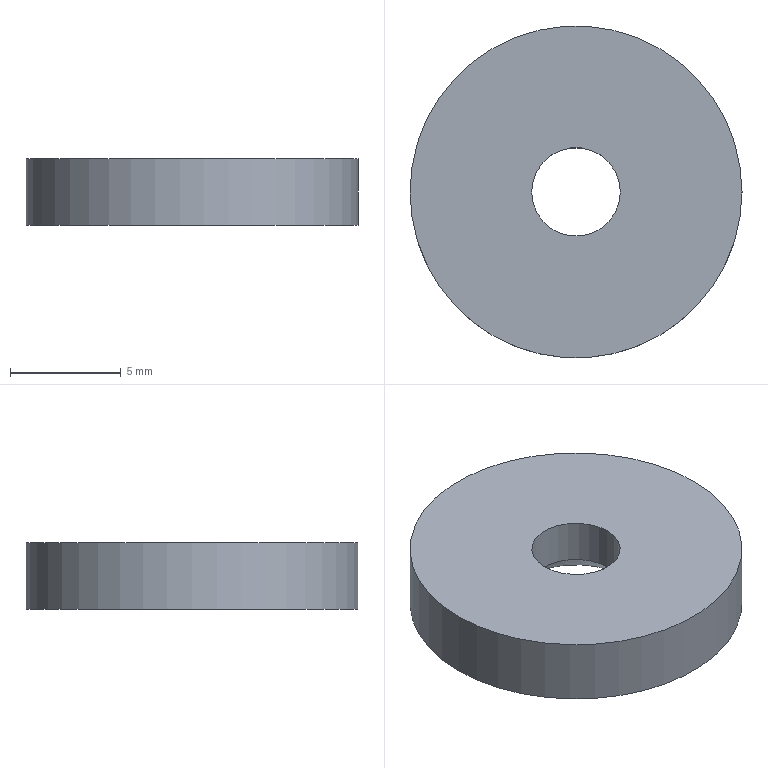Part | NX | features BREP 1, DATUM_CSYS 1 | 1 solid | 5 faces | box 15 x 15 x 3 mm | volume 485.114 mm3 | plane 2 | cylinder 2 | cone 1 | commonest cylinder face diameters 4 x1 15 x1
STEP:
#1=CARTESIAN_POINT('',(7.5,0.,0.));
#2=VERTEX_POINT('',#1);
#3=CARTESIAN_POINT('',(0.,0.,0.));
#4=DIRECTION('',(0.,0.,1.));
#5=DIRECTION('',(1.,0.,0.));
#6=AXIS2_PLACEMENT_3D('',#3,#4,#5);
#7=CIRCLE('',#6,7.5);
#8=EDGE_CURVE('',#2,#2,#7,.T.);
#9=ORIENTED_EDGE('',*,*,#8,.F.);
#10=EDGE_LOOP('',(#9));
#11=FACE_BOUND('',#10,.T.);
#12=CARTESIAN_POINT('',(3.,0.,0.));
#13=VERTEX_POINT('',#12);
#14=CARTESIAN_POINT('',(0.,0.,0.));
#15=DIRECTION('',(0.,0.,1.));
#16=DIRECTION('',(1.,0.,0.));
#17=AXIS2_PLACEMENT_3D('',#14,#15,#16);
#18=CIRCLE('',#17,3.);
#19=EDGE_CURVE('',#13,#13,#18,.T.);
#20=ORIENTED_EDGE('',*,*,#19,.T.);
#21=EDGE_LOOP('',(#20));
#22=FACE_BOUND('',#21,.T.);
#23=CARTESIAN_POINT('',(0.,0.,0.));
#24=DIRECTION('',(0.,0.,1.));
#25=DIRECTION('',(-1.,0.,0.));
#26=AXIS2_PLACEMENT_3D('',#23,#24,#25);
#27=PLANE('',#26);
#28=ADVANCED_FACE('',(#11,#22),#27,.F.);
#29=CARTESIAN_POINT('',(7.5,0.,3.));
#30=VERTEX_POINT('',#29);
#31=CARTESIAN_POINT('',(0.,0.,3.));
#32=DIRECTION('',(0.,0.,1.));
#33=DIRECTION('',(1.,0.,0.));
#34=AXIS2_PLACEMENT_3D('',#31,#32,#33);
#35=CIRCLE('',#34,7.5);
#36=EDGE_CURVE('',#30,#30,#35,.T.);
#37=ORIENTED_EDGE('',*,*,#36,.T.);
#38=EDGE_LOOP('',(#37));
#39=FACE_BOUND('',#38,.T.);
#40=CARTESIAN_POINT('',(2.,0.,3.));
#41=VERTEX_POINT('',#40);
#42=CARTESIAN_POINT('',(0.,0.,3.));
#43=DIRECTION('',(0.,0.,1.));
#44=DIRECTION('',(1.,0.,0.));
#45=AXIS2_PLACEMENT_3D('',#42,#43,#44);
#46=CIRCLE('',#45,2.);
#47=EDGE_CURVE('',#41,#41,#46,.T.);
#48=ORIENTED_EDGE('',*,*,#47,.F.);
#49=EDGE_LOOP('',(#48));
#50=FACE_BOUND('',#49,.T.);
#51=CARTESIAN_POINT('',(0.,0.,3.));
#52=DIRECTION('',(0.,0.,1.));
#53=DIRECTION('',(-1.,0.,0.));
#54=AXIS2_PLACEMENT_3D('',#51,#52,#53);
#55=PLANE('',#54);
#56=ADVANCED_FACE('',(#39,#50),#55,.T.);
#57=ORIENTED_EDGE('',*,*,#8,.T.);
#58=CARTESIAN_POINT('',(7.5,0.,0.));
#59=DIRECTION('',(0.,0.,1.));
#60=VECTOR('',#59,1000.);
#61=LINE('',#58,#60);
#62=EDGE_CURVE('',#2,#30,#61,.T.);
#63=ORIENTED_EDGE('',*,*,#62,.T.);
#64=ORIENTED_EDGE('',*,*,#36,.F.);
#65=ORIENTED_EDGE('',*,*,#62,.F.);
#66=EDGE_LOOP('',(#57,#63,#64,#65));
#67=FACE_BOUND('',#66,.T.);
#68=CARTESIAN_POINT('',(0.,0.,0.));
#69=DIRECTION('',(0.,0.,1.));
#70=DIRECTION('',(-1.,0.,0.));
#71=AXIS2_PLACEMENT_3D('',#68,#69,#70);
#72=CYLINDRICAL_SURFACE('',#71,7.5);
#73=ADVANCED_FACE('',(#67),#72,.T.);
#74=CARTESIAN_POINT('',(2.,0.,1.));
#75=VERTEX_POINT('',#74);
#76=CARTESIAN_POINT('',(3.,0.,0.));
#77=DIRECTION('',(-0.7071,0.,0.7071));
#78=VECTOR('',#77,1000.);
#79=LINE('',#76,#78);
#80=EDGE_CURVE('',#13,#75,#79,.T.);
#81=ORIENTED_EDGE('',*,*,#80,.T.);
#82=CARTESIAN_POINT('',(0.,0.,1.));
#83=DIRECTION('',(0.,0.,1.));
#84=DIRECTION('',(1.,0.,0.));
#85=AXIS2_PLACEMENT_3D('',#82,#83,#84);
#86=CIRCLE('',#85,2.);
#87=EDGE_CURVE('',#75,#75,#86,.T.);
#88=ORIENTED_EDGE('',*,*,#87,.T.);
#89=ORIENTED_EDGE('',*,*,#80,.F.);
#90=ORIENTED_EDGE('',*,*,#19,.F.);
#91=EDGE_LOOP('',(#81,#88,#89,#90));
#92=FACE_BOUND('',#91,.T.);
#93=CARTESIAN_POINT('',(0.,0.,1.));
#94=DIRECTION('',(0.,0.,-1.));
#95=DIRECTION('',(-1.,0.,0.));
#96=AXIS2_PLACEMENT_3D('',#93,#94,#95);
#97=CONICAL_SURFACE('',#96,2.,0.7854);
#98=ADVANCED_FACE('',(#92),#97,.F.);
#99=CARTESIAN_POINT('',(2.,0.,1.));
#100=DIRECTION('',(0.,0.,1.));
#101=VECTOR('',#100,1000.);
#102=LINE('',#99,#101);
#103=EDGE_CURVE('',#75,#41,#102,.T.);
#104=ORIENTED_EDGE('',*,*,#103,.T.);
#105=ORIENTED_EDGE('',*,*,#47,.T.);
#106=ORIENTED_EDGE('',*,*,#103,.F.);
#107=ORIENTED_EDGE('',*,*,#87,.F.);
#108=EDGE_LOOP('',(#104,#105,#106,#107));
#109=FACE_BOUND('',#108,.T.);
#110=CARTESIAN_POINT('',(0.,0.,1.));
#111=DIRECTION('',(0.,0.,1.));
#112=DIRECTION('',(-1.,0.,0.));
#113=AXIS2_PLACEMENT_3D('',#110,#111,#112);
#114=CYLINDRICAL_SURFACE('',#113,2.);
#115=ADVANCED_FACE('',(#109),#114,.F.);
#116=CLOSED_SHELL('',(#28,#56,#73,#98,#115));
#117=MANIFOLD_SOLID_BREP('',#116);
#118=(LENGTH_UNIT()NAMED_UNIT(*)SI_UNIT(.MILLI.,.METRE.));
#119=UNCERTAINTY_MEASURE_WITH_UNIT(LENGTH_MEASURE(0.00001),#118,'','');
#120=(NAMED_UNIT(*)PLANE_ANGLE_UNIT()SI_UNIT($,.RADIAN.));
#121=(NAMED_UNIT(*)SI_UNIT($,.STERADIAN.)SOLID_ANGLE_UNIT());
#122=(GEOMETRIC_REPRESENTATION_CONTEXT(3)GLOBAL_UNCERTAINTY_ASSIGNED_CONTEXT((#119))GLOBAL_UNIT_ASSIGNED_CONTEXT((#118,#120,#121))REPRESENTATION_CONTEXT('',''));
#123=ADVANCED_BREP_SHAPE_REPRESENTATION('',(#117),#122);